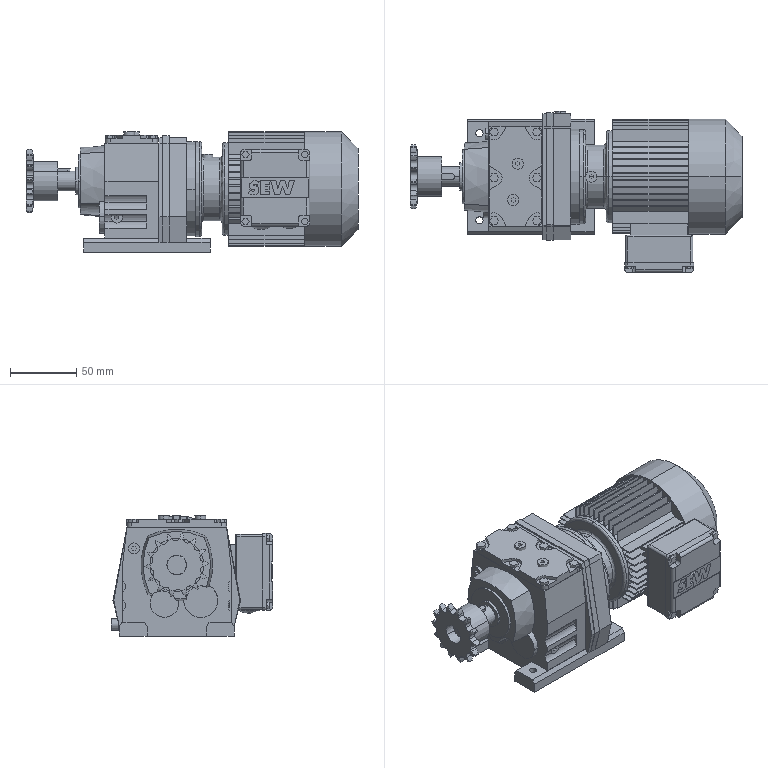Part | STEP file | R37DT71D4 | 19 solids | 810 faces | box 251.513 x 122.1 x 91.448 mm | volume 1177142 mm3 | plane 557 | cylinder 197 | torus 32 | cone 14 | spline 10 | commonest cylinder face diameters 23.409 x30 6.157 x20 4.8 x16 48.615 x15 8.4 x14 3.6 x12